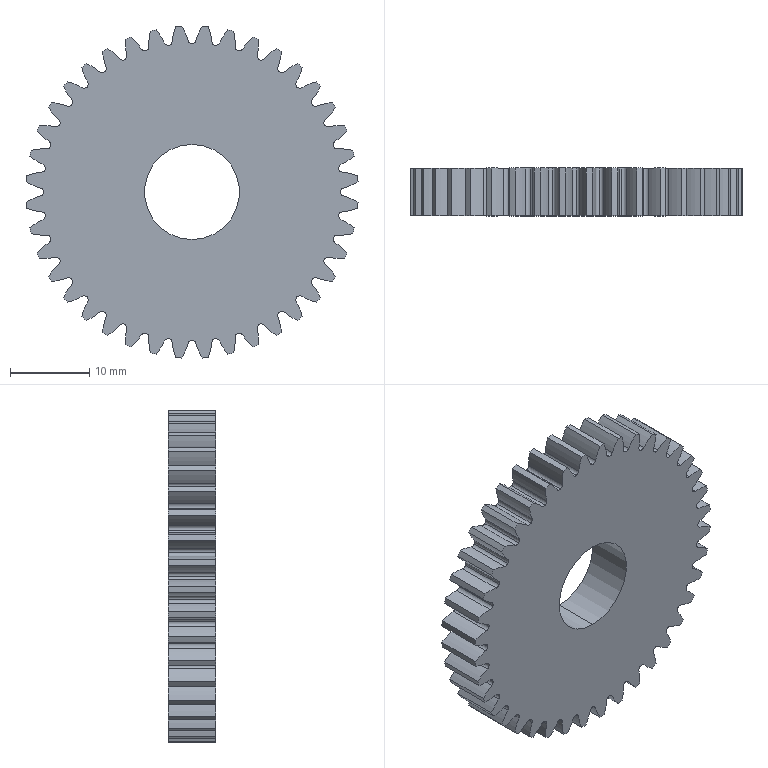Part | SolidWorks | features BaseBody 1, RefAxis 1 | 1 solid | 204 faces | box 41.924 x 6 x 41.924 mm | volume 6820 mm3 | cylinder 202 | plane 2 | commonest cylinder face diameters 1.012 x80 16.21 x80 42 x40 12 x2